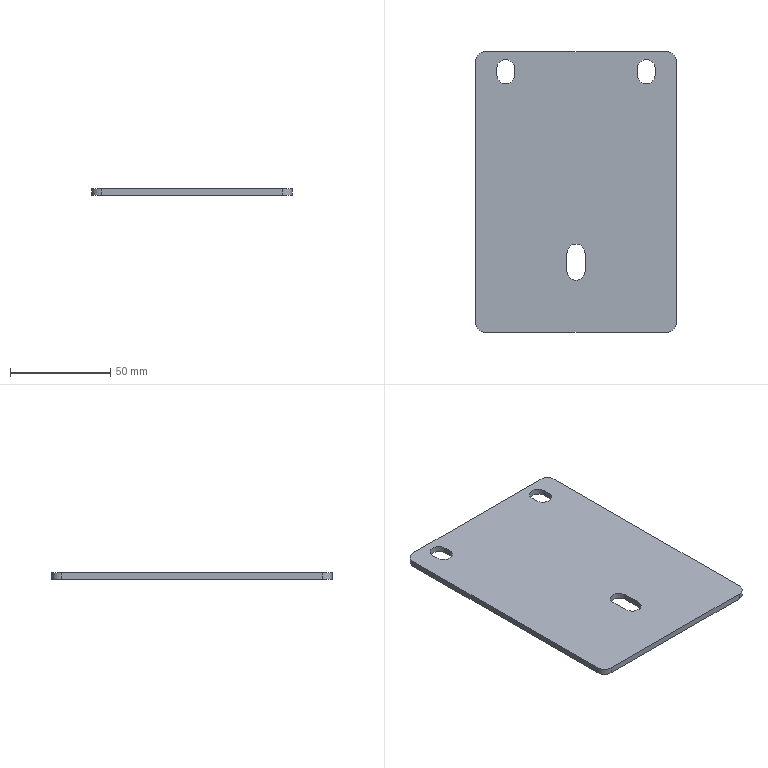Part | STEP file | 6101402 | 1 solid | 22 faces | box 100 x 140 x 3 mm | volume 40958 mm3 | plane 12 | cylinder 10 | commonest cylinder face diameters 9 x6 10 x4